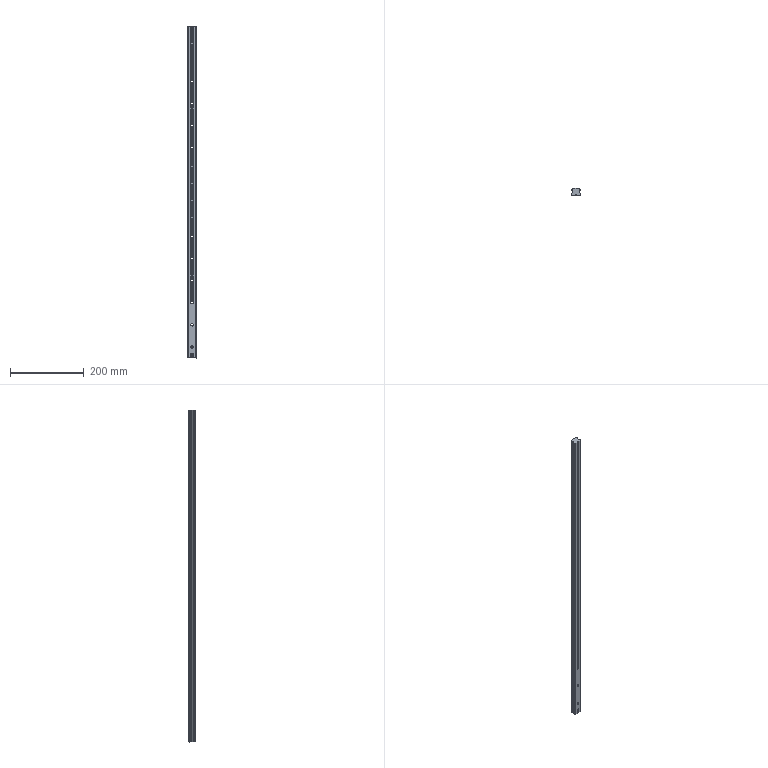Part | SolidWorks | features BaseBody 1, HoleWzd 1, ICE 1, MoveFace 1 | 1 solid | 148 faces | box 23 x 18 x 900 mm | volume 312541 mm3 | plane 80 | cylinder 68 | commonest cylinder face diameters 6.6 x30 11 x30 1 x4 4 x4